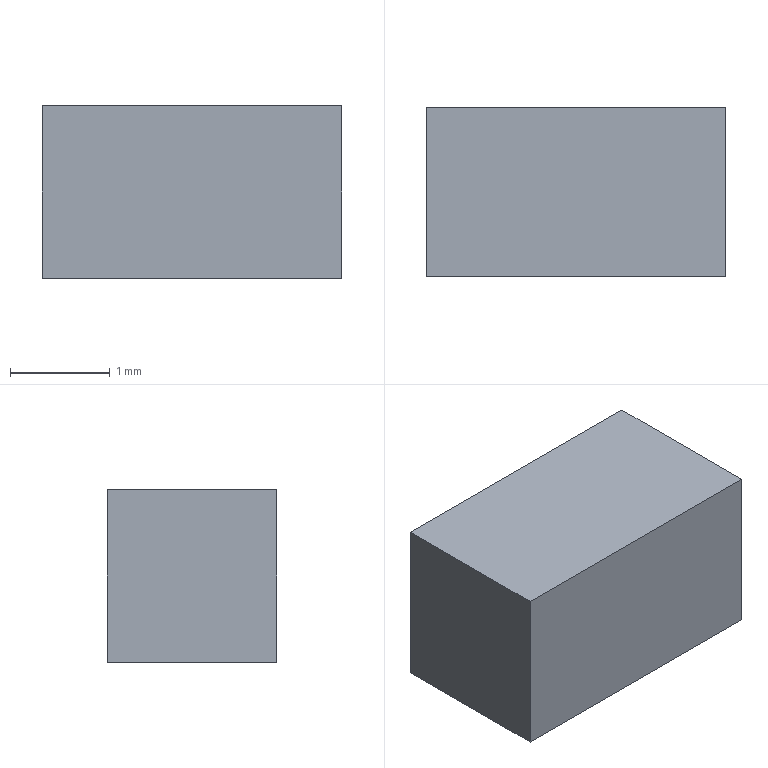Part | Creo | 1 solid | 6 faces | box 3 x 1.7 x 1.724 mm | volume 8.794 mm3 | plane 6
STEP:
#1=CARTESIAN_POINT('',(0.,0.,0.));
#2=DIRECTION('',(0.,0.,1.));
#3=DIRECTION('',(1.,0.,0.));
#4=AXIS2_PLACEMENT_3D('',#1,#2,#3);
#5=CARTESIAN_POINT('',(-1.5,-0.85,0.));
#6=VERTEX_POINT('',#5);
#7=CARTESIAN_POINT('',(1.5,-0.85,0.));
#8=VERTEX_POINT('',#7);
#9=CARTESIAN_POINT('',(-1.5,-0.85,0.));
#10=DIRECTION('',(1.,0.,0.));
#11=VECTOR('',#10,3.);
#12=LINE('',#9,#11);
#13=EDGE_CURVE('',#6,#8,#12,.T.);
#14=ORIENTED_EDGE('',*,*,#13,.T.);
#15=CARTESIAN_POINT('',(1.5,0.85,0.));
#16=VERTEX_POINT('',#15);
#17=CARTESIAN_POINT('',(1.5,-0.85,0.));
#18=DIRECTION('',(0.,1.,0.));
#19=VECTOR('',#18,1.7);
#20=LINE('',#17,#19);
#21=EDGE_CURVE('',#8,#16,#20,.T.);
#22=ORIENTED_EDGE('',*,*,#21,.T.);
#23=CARTESIAN_POINT('',(-1.5,0.85,0.));
#24=VERTEX_POINT('',#23);
#25=CARTESIAN_POINT('',(1.5,0.85,0.));
#26=DIRECTION('',(-1.,0.,0.));
#27=VECTOR('',#26,3.);
#28=LINE('',#25,#27);
#29=EDGE_CURVE('',#16,#24,#28,.T.);
#30=ORIENTED_EDGE('',*,*,#29,.T.);
#31=CARTESIAN_POINT('',(-1.5,0.85,0.));
#32=DIRECTION('',(0.,-1.,0.));
#33=VECTOR('',#32,1.7);
#34=LINE('',#31,#33);
#35=EDGE_CURVE('',#24,#6,#34,.T.);
#36=ORIENTED_EDGE('',*,*,#35,.T.);
#37=EDGE_LOOP('',(#14,#22,#30,#36));
#38=FACE_OUTER_BOUND('',#37,.F.);
#39=CARTESIAN_POINT('',(0.,0.,0.));
#40=DIRECTION('',(0.,0.,1.));
#41=DIRECTION('',(1.,0.,0.));
#42=AXIS2_PLACEMENT_3D('',#39,#40,#41);
#43=PLANE('',#42);
#44=ADVANCED_FACE('',(#38),#43,.F.);
#45=ORIENTED_EDGE('',*,*,#13,.F.);
#46=CARTESIAN_POINT('',(-1.5,-0.85,1.724));
#47=VERTEX_POINT('',#46);
#48=CARTESIAN_POINT('',(-1.5,-0.85,0.));
#49=DIRECTION('',(0.,0.,1.));
#50=VECTOR('',#49,1.724);
#51=LINE('',#48,#50);
#52=EDGE_CURVE('',#6,#47,#51,.T.);
#53=ORIENTED_EDGE('',*,*,#52,.T.);
#54=CARTESIAN_POINT('',(1.5,-0.85,1.724));
#55=VERTEX_POINT('',#54);
#56=CARTESIAN_POINT('',(-1.5,-0.85,1.724));
#57=DIRECTION('',(1.,0.,0.));
#58=VECTOR('',#57,3.);
#59=LINE('',#56,#58);
#60=EDGE_CURVE('',#47,#55,#59,.T.);
#61=ORIENTED_EDGE('',*,*,#60,.T.);
#62=CARTESIAN_POINT('',(1.5,-0.85,0.));
#63=DIRECTION('',(0.,0.,1.));
#64=VECTOR('',#63,1.724);
#65=LINE('',#62,#64);
#66=EDGE_CURVE('',#8,#55,#65,.T.);
#67=ORIENTED_EDGE('',*,*,#66,.F.);
#68=EDGE_LOOP('',(#45,#53,#61,#67));
#69=FACE_OUTER_BOUND('',#68,.F.);
#70=CARTESIAN_POINT('',(-1.5,-0.85,0.));
#71=DIRECTION('',(0.,-1.,0.));
#72=DIRECTION('',(1.,0.,0.));
#73=AXIS2_PLACEMENT_3D('',#70,#71,#72);
#74=PLANE('',#73);
#75=ADVANCED_FACE('',(#69),#74,.T.);
#76=ORIENTED_EDGE('',*,*,#35,.F.);
#77=CARTESIAN_POINT('',(-1.5,0.85,1.724));
#78=VERTEX_POINT('',#77);
#79=CARTESIAN_POINT('',(-1.5,0.85,0.));
#80=DIRECTION('',(0.,0.,1.));
#81=VECTOR('',#80,1.724);
#82=LINE('',#79,#81);
#83=EDGE_CURVE('',#24,#78,#82,.T.);
#84=ORIENTED_EDGE('',*,*,#83,.T.);
#85=CARTESIAN_POINT('',(-1.5,0.85,1.724));
#86=DIRECTION('',(0.,-1.,0.));
#87=VECTOR('',#86,1.7);
#88=LINE('',#85,#87);
#89=EDGE_CURVE('',#78,#47,#88,.T.);
#90=ORIENTED_EDGE('',*,*,#89,.T.);
#91=ORIENTED_EDGE('',*,*,#52,.F.);
#92=EDGE_LOOP('',(#76,#84,#90,#91));
#93=FACE_OUTER_BOUND('',#92,.F.);
#94=CARTESIAN_POINT('',(-1.5,0.85,0.));
#95=DIRECTION('',(-1.,0.,0.));
#96=DIRECTION('',(0.,-1.,0.));
#97=AXIS2_PLACEMENT_3D('',#94,#95,#96);
#98=PLANE('',#97);
#99=ADVANCED_FACE('',(#93),#98,.T.);
#100=ORIENTED_EDGE('',*,*,#29,.F.);
#101=CARTESIAN_POINT('',(1.5,0.85,1.724));
#102=VERTEX_POINT('',#101);
#103=CARTESIAN_POINT('',(1.5,0.85,0.));
#104=DIRECTION('',(0.,0.,1.));
#105=VECTOR('',#104,1.724);
#106=LINE('',#103,#105);
#107=EDGE_CURVE('',#16,#102,#106,.T.);
#108=ORIENTED_EDGE('',*,*,#107,.T.);
#109=CARTESIAN_POINT('',(1.5,0.85,1.724));
#110=DIRECTION('',(-1.,0.,0.));
#111=VECTOR('',#110,3.);
#112=LINE('',#109,#111);
#113=EDGE_CURVE('',#102,#78,#112,.T.);
#114=ORIENTED_EDGE('',*,*,#113,.T.);
#115=ORIENTED_EDGE('',*,*,#83,.F.);
#116=EDGE_LOOP('',(#100,#108,#114,#115));
#117=FACE_OUTER_BOUND('',#116,.F.);
#118=CARTESIAN_POINT('',(1.5,0.85,0.));
#119=DIRECTION('',(0.,1.,0.));
#120=DIRECTION('',(-1.,0.,0.));
#121=AXIS2_PLACEMENT_3D('',#118,#119,#120);
#122=PLANE('',#121);
#123=ADVANCED_FACE('',(#117),#122,.T.);
#124=ORIENTED_EDGE('',*,*,#21,.F.);
#125=ORIENTED_EDGE('',*,*,#66,.T.);
#126=CARTESIAN_POINT('',(1.5,-0.85,1.724));
#127=DIRECTION('',(0.,1.,0.));
#128=VECTOR('',#127,1.7);
#129=LINE('',#126,#128);
#130=EDGE_CURVE('',#55,#102,#129,.T.);
#131=ORIENTED_EDGE('',*,*,#130,.T.);
#132=ORIENTED_EDGE('',*,*,#107,.F.);
#133=EDGE_LOOP('',(#124,#125,#131,#132));
#134=FACE_OUTER_BOUND('',#133,.F.);
#135=CARTESIAN_POINT('',(1.5,-0.85,0.));
#136=DIRECTION('',(1.,0.,0.));
#137=DIRECTION('',(0.,1.,0.));
#138=AXIS2_PLACEMENT_3D('',#135,#136,#137);
#139=PLANE('',#138);
#140=ADVANCED_FACE('',(#134),#139,.T.);
#141=ORIENTED_EDGE('',*,*,#60,.F.);
#142=ORIENTED_EDGE('',*,*,#89,.F.);
#143=ORIENTED_EDGE('',*,*,#113,.F.);
#144=ORIENTED_EDGE('',*,*,#130,.F.);
#145=EDGE_LOOP('',(#141,#142,#143,#144));
#146=FACE_OUTER_BOUND('',#145,.F.);
#147=CARTESIAN_POINT('',(0.,0.,1.724));
#148=DIRECTION('',(0.,0.,1.));
#149=DIRECTION('',(1.,0.,0.));
#150=AXIS2_PLACEMENT_3D('',#147,#148,#149);
#151=PLANE('',#150);
#152=ADVANCED_FACE('',(#146),#151,.T.);
#153=CLOSED_SHELL('',(#44,#75,#99,#123,#140,#152));
#154=MANIFOLD_SOLID_BREP('',#153);
#155=(LENGTH_UNIT()NAMED_UNIT(*)SI_UNIT(.MILLI.,.METRE.));
#156=UNCERTAINTY_MEASURE_WITH_UNIT(LENGTH_MEASURE(0.0003855),#155,'','');
#157=(NAMED_UNIT(*)PLANE_ANGLE_UNIT()SI_UNIT($,.RADIAN.));
#158=PLANE_ANGLE_MEASURE_WITH_UNIT(PLANE_ANGLE_MEASURE(0.01745),#157);
#159=(CONVERSION_BASED_UNIT('DEGREE',#158)NAMED_UNIT(*)PLANE_ANGLE_UNIT());
#160=(NAMED_UNIT(*)SI_UNIT($,.STERADIAN.)SOLID_ANGLE_UNIT());
#161=(GEOMETRIC_REPRESENTATION_CONTEXT(3)GLOBAL_UNCERTAINTY_ASSIGNED_CONTEXT((#156))GLOBAL_UNIT_ASSIGNED_CONTEXT((#155,#159,#160))REPRESENTATION_CONTEXT('',''));
#162=ADVANCED_BREP_SHAPE_REPRESENTATION('',(#4,#154),#161);